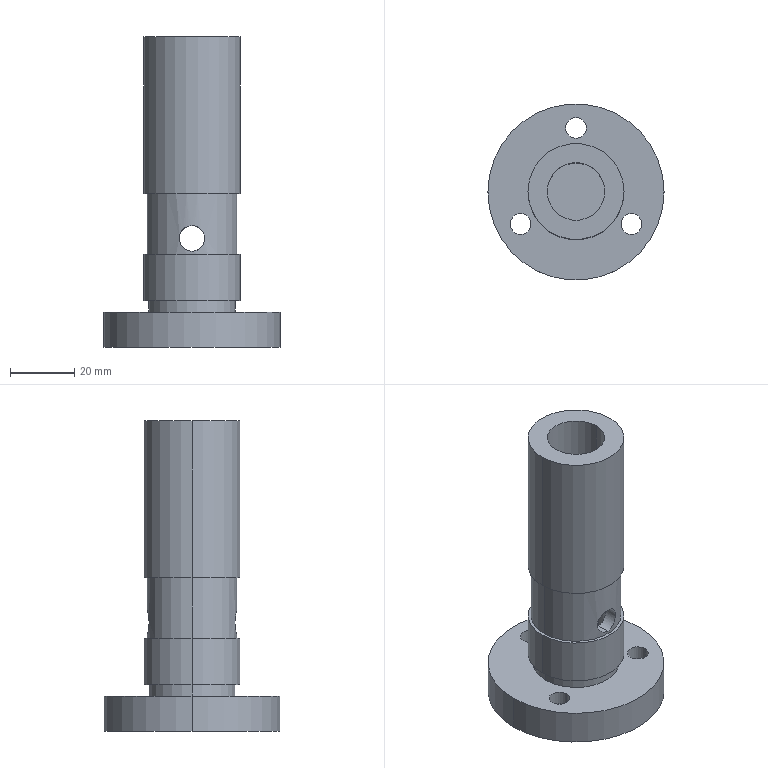Part | SolidWorks | features ICE 9, CirPattern 1, Extrusion 1 | 1 solid | 41 faces | box 55 x 55 x 97 mm | volume 56843 mm3 | cylinder 30 | plane 11 | commonest cylinder face diameters 6.5 x6 11 x6 8 x4 30 x4 18 x2 20 x2
STEP:
#1=CARTESIAN_POINT('',(0.,-14.,30.));
#2=VERTEX_POINT('',#1);
#3=CARTESIAN_POINT('',(0.,-14.,38.));
#4=VERTEX_POINT('',#3);
#5=CARTESIAN_POINT('',(0.,-14.,30.));
#6=CARTESIAN_POINT('',(-0.2619,-14.,30.));
#7=CARTESIAN_POINT('',(-0.524,-13.993,30.026));
#8=CARTESIAN_POINT('',(-1.043,-13.963,30.129));
#9=CARTESIAN_POINT('',(-1.294,-13.942,30.206));
#10=CARTESIAN_POINT('',(-1.776,-13.889,30.406));
#11=CARTESIAN_POINT('',(-2.01,-13.857,30.532));
#12=CARTESIAN_POINT('',(-2.443,-13.787,30.822));
#13=CARTESIAN_POINT('',(-2.643,-13.749,30.987));
#14=CARTESIAN_POINT('',(-3.012,-13.673,31.355));
#15=CARTESIAN_POINT('',(-3.18,-13.635,31.559));
#16=CARTESIAN_POINT('',(-3.468,-13.564,31.991));
#17=CARTESIAN_POINT('',(-3.592,-13.532,32.22));
#18=CARTESIAN_POINT('',(-3.795,-13.476,32.708));
#19=CARTESIAN_POINT('',(-3.871,-13.454,32.958));
#20=CARTESIAN_POINT('',(-3.973,-13.424,33.47));
#21=CARTESIAN_POINT('',(-4.,-13.416,33.736));
#22=CARTESIAN_POINT('',(-4.,-13.416,34.263));
#23=CARTESIAN_POINT('',(-3.974,-13.424,34.524));
#24=CARTESIAN_POINT('',(-3.872,-13.454,35.038));
#25=CARTESIAN_POINT('',(-3.794,-13.477,35.294));
#26=CARTESIAN_POINT('',(-3.594,-13.531,35.776));
#27=CARTESIAN_POINT('',(-3.471,-13.564,36.005));
#28=CARTESIAN_POINT('',(-3.179,-13.635,36.442));
#29=CARTESIAN_POINT('',(-3.013,-13.673,36.644));
#30=CARTESIAN_POINT('',(-2.646,-13.749,37.011));
#31=CARTESIAN_POINT('',(-2.443,-13.787,37.178));
#32=CARTESIAN_POINT('',(-2.008,-13.857,37.469));
#33=CARTESIAN_POINT('',(-1.779,-13.889,37.592));
#34=CARTESIAN_POINT('',(-1.297,-13.942,37.793));
#35=CARTESIAN_POINT('',(-1.042,-13.964,37.871));
#36=CARTESIAN_POINT('',(-0.5273,-13.992,37.974));
#37=CARTESIAN_POINT('',(-0.2657,-14.,38.));
#38=CARTESIAN_POINT('',(0.,-14.,38.));
#39=B_SPLINE_CURVE_WITH_KNOTS('',3,(#5,#6,#7,#8,#9,#10,#11,#12,#13,#14,#15,#16,#17,#18,#19,#20,#21,#22,#23,#24,#25,#26,#27,#28,#29,#30,#31,#32,#33,#34,#35,#36,#37,#38),.UNSPECIFIED.,.F.,.F.,(4,2,2,2,2,2,2,2,2,2,2,2,2,2,2,2,4),(0.01257,0.01336,0.01414,0.01493,0.01571,0.0165,0.01728,0.01807,0.01886,0.01964,0.02043,0.02121,0.022,0.02278,0.02357,0.02435,0.02514),.UNSPECIFIED.);
#40=EDGE_CURVE('',#2,#4,#39,.T.);
#41=ORIENTED_EDGE('',*,*,#40,.F.);
#42=CARTESIAN_POINT('',(0.,-10.,30.));
#43=VERTEX_POINT('',#42);
#44=CARTESIAN_POINT('',(0.,-26.75,30.));
#45=DIRECTION('',(0.,1.,0.));
#46=VECTOR('',#45,1000.);
#47=LINE('',#44,#46);
#48=EDGE_CURVE('',#2,#43,#47,.T.);
#49=ORIENTED_EDGE('',*,*,#48,.T.);
#50=CARTESIAN_POINT('',(0.,-10.,38.));
#51=VERTEX_POINT('',#50);
#52=CARTESIAN_POINT('',(0.,-10.,38.));
#53=CARTESIAN_POINT('',(-0.2673,-10.,38.));
#54=CARTESIAN_POINT('',(-0.5296,-9.989,37.973));
#55=CARTESIAN_POINT('',(-1.045,-9.949,37.87));
#56=CARTESIAN_POINT('',(-1.3,-9.918,37.792));
#57=CARTESIAN_POINT('',(-1.784,-9.843,37.59));
#58=CARTESIAN_POINT('',(-2.013,-9.798,37.467));
#59=CARTESIAN_POINT('',(-2.445,-9.699,37.176));
#60=CARTESIAN_POINT('',(-2.648,-9.645,37.009));
#61=CARTESIAN_POINT('',(-3.013,-9.537,36.644));
#62=CARTESIAN_POINT('',(-3.178,-9.483,36.444));
#63=CARTESIAN_POINT('',(-3.469,-9.38,36.009));
#64=CARTESIAN_POINT('',(-3.591,-9.333,35.78));
#65=CARTESIAN_POINT('',(-3.792,-9.254,35.3));
#66=CARTESIAN_POINT('',(-3.87,-9.221,35.046));
#67=CARTESIAN_POINT('',(-3.974,-9.177,34.528));
#68=CARTESIAN_POINT('',(-4.,-9.165,34.267));
#69=CARTESIAN_POINT('',(-4.,-9.165,33.738));
#70=CARTESIAN_POINT('',(-3.973,-9.177,33.47));
#71=CARTESIAN_POINT('',(-3.87,-9.221,32.955));
#72=CARTESIAN_POINT('',(-3.793,-9.253,32.703));
#73=CARTESIAN_POINT('',(-3.59,-9.334,32.216));
#74=CARTESIAN_POINT('',(-3.466,-9.381,31.987));
#75=CARTESIAN_POINT('',(-3.178,-9.483,31.557));
#76=CARTESIAN_POINT('',(-3.01,-9.538,31.354));
#77=CARTESIAN_POINT('',(-2.644,-9.646,30.988));
#78=CARTESIAN_POINT('',(-2.445,-9.699,30.824));
#79=CARTESIAN_POINT('',(-2.013,-9.798,30.534));
#80=CARTESIAN_POINT('',(-1.78,-9.843,30.408));
#81=CARTESIAN_POINT('',(-1.299,-9.918,30.208));
#82=CARTESIAN_POINT('',(-1.049,-9.948,30.131));
#83=CARTESIAN_POINT('',(-0.5273,-9.99,30.026));
#84=CARTESIAN_POINT('',(-0.2633,-10.,30.));
#85=CARTESIAN_POINT('',(0.,-10.,30.));
#86=B_SPLINE_CURVE_WITH_KNOTS('',3,(#52,#53,#54,#55,#56,#57,#58,#59,#60,#61,#62,#63,#64,#65,#66,#67,#68,#69,#70,#71,#72,#73,#74,#75,#76,#77,#78,#79,#80,#81,#82,#83,#84,#85),.UNSPECIFIED.,.F.,.F.,(4,2,2,2,2,2,2,2,2,2,2,2,2,2,2,2,4),(0.,0.00079,0.00158,0.00237,0.00316,0.00395,0.00474,0.00553,0.00632,0.00711,0.0079,0.00869,0.00948,0.01027,0.01106,0.01185,0.01264),.UNSPECIFIED.);
#87=EDGE_CURVE('',#51,#43,#86,.T.);
#88=ORIENTED_EDGE('',*,*,#87,.F.);
#89=CARTESIAN_POINT('',(0.,-26.75,38.));
#90=DIRECTION('',(0.,1.,0.));
#91=VECTOR('',#90,1000.);
#92=LINE('',#89,#91);
#93=EDGE_CURVE('',#4,#51,#92,.T.);
#94=ORIENTED_EDGE('',*,*,#93,.F.);
#95=EDGE_LOOP('',(#41,#49,#88,#94));
#96=FACE_OUTER_BOUND('',#95,.T.);
#97=CARTESIAN_POINT('',(0.,-26.75,34.));
#98=DIRECTION('',(0.,1.,0.));
#99=DIRECTION('',(0.,0.,1.));
#100=AXIS2_PLACEMENT_3D('',#97,#98,#99);
#101=CYLINDRICAL_SURFACE('',#100,4.);
#102=ADVANCED_FACE('',(#96),#101,.F.);
#103=CARTESIAN_POINT('',(0.,10.,30.));
#104=VERTEX_POINT('',#103);
#105=CARTESIAN_POINT('',(0.,10.,38.));
#106=VERTEX_POINT('',#105);
#107=CARTESIAN_POINT('',(0.,10.,30.));
#108=CARTESIAN_POINT('',(-0.2631,10.,30.));
#109=CARTESIAN_POINT('',(-0.5298,9.989,30.026));
#110=CARTESIAN_POINT('',(-1.048,9.948,30.131));
#111=CARTESIAN_POINT('',(-1.299,9.918,30.208));
#112=CARTESIAN_POINT('',(-1.782,9.843,30.409));
#113=CARTESIAN_POINT('',(-2.015,9.797,30.535));
#114=CARTESIAN_POINT('',(-2.446,9.699,30.824));
#115=CARTESIAN_POINT('',(-2.646,9.645,30.989));
#116=CARTESIAN_POINT('',(-3.015,9.537,31.358));
#117=CARTESIAN_POINT('',(-3.179,9.483,31.558));
#118=CARTESIAN_POINT('',(-3.466,9.381,31.987));
#119=CARTESIAN_POINT('',(-3.592,9.333,32.22));
#120=CARTESIAN_POINT('',(-3.793,9.253,32.703));
#121=CARTESIAN_POINT('',(-3.869,9.221,32.952));
#122=CARTESIAN_POINT('',(-3.973,9.177,33.468));
#123=CARTESIAN_POINT('',(-4.,9.165,33.736));
#124=CARTESIAN_POINT('',(-4.,9.165,34.263));
#125=CARTESIAN_POINT('',(-3.974,9.177,34.525));
#126=CARTESIAN_POINT('',(-3.87,9.221,35.046));
#127=CARTESIAN_POINT('',(-3.792,9.254,35.298));
#128=CARTESIAN_POINT('',(-3.592,9.333,35.78));
#129=CARTESIAN_POINT('',(-3.467,9.381,36.013));
#130=CARTESIAN_POINT('',(-3.177,9.483,36.444));
#131=CARTESIAN_POINT('',(-3.013,9.537,36.644));
#132=CARTESIAN_POINT('',(-2.646,9.645,37.011));
#133=CARTESIAN_POINT('',(-2.443,9.699,37.178));
#134=CARTESIAN_POINT('',(-2.014,9.798,37.466));
#135=CARTESIAN_POINT('',(-1.785,9.842,37.589));
#136=CARTESIAN_POINT('',(-1.298,9.918,37.793));
#137=CARTESIAN_POINT('',(-1.046,9.948,37.87));
#138=CARTESIAN_POINT('',(-0.5323,9.989,37.973));
#139=CARTESIAN_POINT('',(-0.2671,10.,38.));
#140=CARTESIAN_POINT('',(0.,10.,38.));
#141=B_SPLINE_CURVE_WITH_KNOTS('',3,(#107,#108,#109,#110,#111,#112,#113,#114,#115,#116,#117,#118,#119,#120,#121,#122,#123,#124,#125,#126,#127,#128,#129,#130,#131,#132,#133,#134,#135,#136,#137,#138,#139,#140),.UNSPECIFIED.,.F.,.F.,(4,2,2,2,2,2,2,2,2,2,2,2,2,2,2,2,4),(0.01264,0.01343,0.01422,0.01501,0.0158,0.01659,0.01738,0.01817,0.01896,0.01974,0.02053,0.02132,0.02211,0.0229,0.02369,0.02448,0.02527),.UNSPECIFIED.);
#142=EDGE_CURVE('',#104,#106,#141,.T.);
#143=ORIENTED_EDGE('',*,*,#142,.F.);
#144=CARTESIAN_POINT('',(0.,14.,30.));
#145=VERTEX_POINT('',#144);
#146=CARTESIAN_POINT('',(0.,-26.75,30.));
#147=DIRECTION('',(0.,1.,0.));
#148=VECTOR('',#147,1000.);
#149=LINE('',#146,#148);
#150=EDGE_CURVE('',#104,#145,#149,.T.);
#151=ORIENTED_EDGE('',*,*,#150,.T.);
#152=CARTESIAN_POINT('',(0.,14.,38.));
#153=VERTEX_POINT('',#152);
#154=CARTESIAN_POINT('',(0.,14.,38.));
#155=CARTESIAN_POINT('',(-0.2658,14.,38.));
#156=CARTESIAN_POINT('',(-0.5269,13.992,37.974));
#157=CARTESIAN_POINT('',(-1.04,13.964,37.871));
#158=CARTESIAN_POINT('',(-1.295,13.942,37.794));
#159=CARTESIAN_POINT('',(-1.779,13.889,37.592));
#160=CARTESIAN_POINT('',(-2.008,13.857,37.469));
#161=CARTESIAN_POINT('',(-2.442,13.787,37.179));
#162=CARTESIAN_POINT('',(-2.646,13.749,37.011));
#163=CARTESIAN_POINT('',(-3.013,13.673,36.644));
#164=CARTESIAN_POINT('',(-3.178,13.635,36.443));
#165=CARTESIAN_POINT('',(-3.47,13.564,36.007));
#166=CARTESIAN_POINT('',(-3.594,13.531,35.776));
#167=CARTESIAN_POINT('',(-3.793,13.477,35.295));
#168=CARTESIAN_POINT('',(-3.871,13.454,35.042));
#169=CARTESIAN_POINT('',(-3.974,13.424,34.525));
#170=CARTESIAN_POINT('',(-4.,13.416,34.264));
#171=CARTESIAN_POINT('',(-4.,13.416,33.739));
#172=CARTESIAN_POINT('',(-3.974,13.424,33.473));
#173=CARTESIAN_POINT('',(-3.871,13.454,32.958));
#174=CARTESIAN_POINT('',(-3.795,13.476,32.708));
#175=CARTESIAN_POINT('',(-3.593,13.532,32.222));
#176=CARTESIAN_POINT('',(-3.468,13.564,31.991));
#177=CARTESIAN_POINT('',(-3.179,13.635,31.559));
#178=CARTESIAN_POINT('',(-3.012,13.673,31.355));
#179=CARTESIAN_POINT('',(-2.643,13.75,30.986));
#180=CARTESIAN_POINT('',(-2.442,13.787,30.821));
#181=CARTESIAN_POINT('',(-2.01,13.857,30.532));
#182=CARTESIAN_POINT('',(-1.776,13.889,30.406));
#183=CARTESIAN_POINT('',(-1.293,13.942,30.206));
#184=CARTESIAN_POINT('',(-1.044,13.963,30.13));
#185=CARTESIAN_POINT('',(-0.5274,13.992,30.026));
#186=CARTESIAN_POINT('',(-0.2619,14.,30.));
#187=CARTESIAN_POINT('',(0.,14.,30.));
#188=B_SPLINE_CURVE_WITH_KNOTS('',3,(#154,#155,#156,#157,#158,#159,#160,#161,#162,#163,#164,#165,#166,#167,#168,#169,#170,#171,#172,#173,#174,#175,#176,#177,#178,#179,#180,#181,#182,#183,#184,#185,#186,#187),.UNSPECIFIED.,.F.,.F.,(4,2,2,2,2,2,2,2,2,2,2,2,2,2,2,2,4),(0.,0.0007857,0.001571,0.002357,0.003143,0.003929,0.004714,0.0055,0.006286,0.007072,0.007857,0.008643,0.009429,0.01021,0.011,0.01179,0.01257),.UNSPECIFIED.);
#189=EDGE_CURVE('',#153,#145,#188,.T.);
#190=ORIENTED_EDGE('',*,*,#189,.F.);
#191=CARTESIAN_POINT('',(0.,-26.75,38.));
#192=DIRECTION('',(0.,1.,0.));
#193=VECTOR('',#192,1000.);
#194=LINE('',#191,#193);
#195=EDGE_CURVE('',#106,#153,#194,.T.);
#196=ORIENTED_EDGE('',*,*,#195,.F.);
#197=EDGE_LOOP('',(#143,#151,#190,#196));
#198=FACE_OUTER_BOUND('',#197,.T.);
#199=CARTESIAN_POINT('',(0.,-26.75,34.));
#200=DIRECTION('',(0.,1.,0.));
#201=DIRECTION('',(0.,0.,1.));
#202=AXIS2_PLACEMENT_3D('',#199,#200,#201);
#203=CYLINDRICAL_SURFACE('',#202,4.);
#204=ADVANCED_FACE('',(#198),#203,.F.);
#205=CARTESIAN_POINT('',(-20.571,-10.,11.));
#206=VERTEX_POINT('',#205);
#207=CARTESIAN_POINT('',(-14.071,-10.,11.));
#208=VERTEX_POINT('',#207);
#209=CARTESIAN_POINT('',(-17.321,-10.,11.));
#210=DIRECTION('',(0.,0.,1.));
#211=DIRECTION('',(1.,0.,0.));
#212=AXIS2_PLACEMENT_3D('',#209,#210,#211);
#213=CIRCLE('',#212,3.25);
#214=EDGE_CURVE('',#206,#208,#213,.T.);
#215=ORIENTED_EDGE('',*,*,#214,.T.);
#216=CARTESIAN_POINT('',(-14.071,-10.,6.5));
#217=VERTEX_POINT('',#216);
#218=CARTESIAN_POINT('',(-14.071,-10.,13.));
#219=DIRECTION('',(0.,0.,-1.));
#220=VECTOR('',#219,1000.);
#221=LINE('',#218,#220);
#222=EDGE_CURVE('',#208,#217,#221,.T.);
#223=ORIENTED_EDGE('',*,*,#222,.T.);
#224=CARTESIAN_POINT('',(-20.571,-10.,6.5));
#225=VERTEX_POINT('',#224);
#226=CARTESIAN_POINT('',(-17.321,-10.,6.5));
#227=DIRECTION('',(0.,0.,-1.));
#228=DIRECTION('',(0.5,-0.866,0.));
#229=AXIS2_PLACEMENT_3D('',#226,#227,#228);
#230=CIRCLE('',#229,3.25);
#231=EDGE_CURVE('',#217,#225,#230,.T.);
#232=ORIENTED_EDGE('',*,*,#231,.T.);
#233=CARTESIAN_POINT('',(-20.571,-10.,13.));
#234=DIRECTION('',(0.,0.,-1.));
#235=VECTOR('',#234,1000.);
#236=LINE('',#233,#235);
#237=EDGE_CURVE('',#206,#225,#236,.T.);
#238=ORIENTED_EDGE('',*,*,#237,.F.);
#239=EDGE_LOOP('',(#215,#223,#232,#238));
#240=FACE_OUTER_BOUND('',#239,.T.);
#241=CARTESIAN_POINT('',(-17.321,-10.,13.));
#242=DIRECTION('',(0.,0.,-1.));
#243=DIRECTION('',(-1.,0.,0.));
#244=AXIS2_PLACEMENT_3D('',#241,#242,#243);
#245=CYLINDRICAL_SURFACE('',#244,3.25);
#246=ADVANCED_FACE('',(#240),#245,.F.);
#247=CARTESIAN_POINT('',(14.071,-10.,11.));
#248=VERTEX_POINT('',#247);
#249=CARTESIAN_POINT('',(20.571,-10.,11.));
#250=VERTEX_POINT('',#249);
#251=CARTESIAN_POINT('',(17.321,-10.,11.));
#252=DIRECTION('',(0.,0.,1.));
#253=DIRECTION('',(1.,0.,0.));
#254=AXIS2_PLACEMENT_3D('',#251,#252,#253);
#255=CIRCLE('',#254,3.25);
#256=EDGE_CURVE('',#248,#250,#255,.T.);
#257=ORIENTED_EDGE('',*,*,#256,.T.);
#258=CARTESIAN_POINT('',(20.571,-10.,6.5));
#259=VERTEX_POINT('',#258);
#260=CARTESIAN_POINT('',(20.571,-10.,13.));
#261=DIRECTION('',(0.,0.,-1.));
#262=VECTOR('',#261,1000.);
#263=LINE('',#260,#262);
#264=EDGE_CURVE('',#250,#259,#263,.T.);
#265=ORIENTED_EDGE('',*,*,#264,.T.);
#266=CARTESIAN_POINT('',(14.071,-10.,6.5));
#267=VERTEX_POINT('',#266);
#268=CARTESIAN_POINT('',(17.321,-10.,6.5));
#269=DIRECTION('',(0.,0.,-1.));
#270=DIRECTION('',(0.5,0.866,0.));
#271=AXIS2_PLACEMENT_3D('',#268,#269,#270);
#272=CIRCLE('',#271,3.25);
#273=EDGE_CURVE('',#259,#267,#272,.T.);
#274=ORIENTED_EDGE('',*,*,#273,.T.);
#275=CARTESIAN_POINT('',(14.071,-10.,13.));
#276=DIRECTION('',(0.,0.,-1.));
#277=VECTOR('',#276,1000.);
#278=LINE('',#275,#277);
#279=EDGE_CURVE('',#248,#267,#278,.T.);
#280=ORIENTED_EDGE('',*,*,#279,.F.);
#281=EDGE_LOOP('',(#257,#265,#274,#280));
#282=FACE_OUTER_BOUND('',#281,.T.);
#283=CARTESIAN_POINT('',(17.321,-10.,13.));
#284=DIRECTION('',(0.,0.,-1.));
#285=DIRECTION('',(-1.,0.,0.));
#286=AXIS2_PLACEMENT_3D('',#283,#284,#285);
#287=CYLINDRICAL_SURFACE('',#286,3.25);
#288=ADVANCED_FACE('',(#282),#287,.F.);
#289=CARTESIAN_POINT('',(-11.821,-10.,6.5));
#290=VERTEX_POINT('',#289);
#291=CARTESIAN_POINT('',(-22.821,-10.,6.5));
#292=VERTEX_POINT('',#291);
#293=CARTESIAN_POINT('',(-17.321,-10.,6.5));
#294=DIRECTION('',(0.,0.,-1.));
#295=DIRECTION('',(0.5,-0.866,0.));
#296=AXIS2_PLACEMENT_3D('',#293,#294,#295);
#297=CIRCLE('',#296,5.5);
#298=EDGE_CURVE('',#290,#292,#297,.T.);
#299=ORIENTED_EDGE('',*,*,#298,.F.);
#300=CARTESIAN_POINT('',(-11.821,-10.,0.));
#301=VERTEX_POINT('',#300);
#302=CARTESIAN_POINT('',(-11.821,-10.,6.5));
#303=DIRECTION('',(0.,0.,-1.));
#304=VECTOR('',#303,1000.);
#305=LINE('',#302,#304);
#306=EDGE_CURVE('',#290,#301,#305,.T.);
#307=ORIENTED_EDGE('',*,*,#306,.T.);
#308=CARTESIAN_POINT('',(-22.821,-10.,0.));
#309=VERTEX_POINT('',#308);
#310=CARTESIAN_POINT('',(-17.321,-10.,0.));
#311=DIRECTION('',(0.,0.,-1.));
#312=DIRECTION('',(0.5,-0.866,0.));
#313=AXIS2_PLACEMENT_3D('',#310,#311,#312);
#314=CIRCLE('',#313,5.5);
#315=EDGE_CURVE('',#301,#309,#314,.T.);
#316=ORIENTED_EDGE('',*,*,#315,.T.);
#317=CARTESIAN_POINT('',(-22.821,-10.,6.5));
#318=DIRECTION('',(0.,0.,-1.));
#319=VECTOR('',#318,1000.);
#320=LINE('',#317,#319);
#321=EDGE_CURVE('',#292,#309,#320,.T.);
#322=ORIENTED_EDGE('',*,*,#321,.F.);
#323=EDGE_LOOP('',(#299,#307,#316,#322));
#324=FACE_OUTER_BOUND('',#323,.T.);
#325=CARTESIAN_POINT('',(-17.321,-10.,6.5));
#326=DIRECTION('',(0.,0.,-1.));
#327=DIRECTION('',(-1.,0.,0.));
#328=AXIS2_PLACEMENT_3D('',#325,#326,#327);
#329=CYLINDRICAL_SURFACE('',#328,5.5);
#330=ADVANCED_FACE('',(#324),#329,.F.);
#331=CARTESIAN_POINT('',(22.821,-10.,6.5));
#332=VERTEX_POINT('',#331);
#333=CARTESIAN_POINT('',(11.821,-10.,6.5));
#334=VERTEX_POINT('',#333);
#335=CARTESIAN_POINT('',(17.321,-10.,6.5));
#336=DIRECTION('',(0.,0.,-1.));
#337=DIRECTION('',(0.5,0.866,0.));
#338=AXIS2_PLACEMENT_3D('',#335,#336,#337);
#339=CIRCLE('',#338,5.5);
#340=EDGE_CURVE('',#332,#334,#339,.T.);
#341=ORIENTED_EDGE('',*,*,#340,.F.);
#342=CARTESIAN_POINT('',(22.821,-10.,0.));
#343=VERTEX_POINT('',#342);
#344=CARTESIAN_POINT('',(22.821,-10.,6.5));
#345=DIRECTION('',(0.,0.,-1.));
#346=VECTOR('',#345,1000.);
#347=LINE('',#344,#346);
#348=EDGE_CURVE('',#332,#343,#347,.T.);
#349=ORIENTED_EDGE('',*,*,#348,.T.);
#350=CARTESIAN_POINT('',(11.821,-10.,0.));
#351=VERTEX_POINT('',#350);
#352=CARTESIAN_POINT('',(17.321,-10.,0.));
#353=DIRECTION('',(0.,0.,-1.));
#354=DIRECTION('',(0.5,0.866,0.));
#355=AXIS2_PLACEMENT_3D('',#352,#353,#354);
#356=CIRCLE('',#355,5.5);
#357=EDGE_CURVE('',#343,#351,#356,.T.);
#358=ORIENTED_EDGE('',*,*,#357,.T.);
#359=CARTESIAN_POINT('',(11.821,-10.,6.5));
#360=DIRECTION('',(0.,0.,-1.));
#361=VECTOR('',#360,1000.);
#362=LINE('',#359,#361);
#363=EDGE_CURVE('',#334,#351,#362,.T.);
#364=ORIENTED_EDGE('',*,*,#363,.F.);
#365=EDGE_LOOP('',(#341,#349,#358,#364));
#366=FACE_OUTER_BOUND('',#365,.T.);
#367=CARTESIAN_POINT('',(17.321,-10.,6.5));
#368=DIRECTION('',(0.,0.,-1.));
#369=DIRECTION('',(-1.,0.,0.));
#370=AXIS2_PLACEMENT_3D('',#367,#368,#369);
#371=CYLINDRICAL_SURFACE('',#370,5.5);
#372=ADVANCED_FACE('',(#366),#371,.F.);
#373=CARTESIAN_POINT('',(-3.25,20.,11.));
#374=VERTEX_POINT('',#373);
#375=CARTESIAN_POINT('',(3.25,20.,11.));
#376=VERTEX_POINT('',#375);
#377=CARTESIAN_POINT('',(0.,20.,11.));
#378=DIRECTION('',(0.,0.,1.));
#379=DIRECTION('',(1.,0.,0.));
#380=AXIS2_PLACEMENT_3D('',#377,#378,#379);
#381=CIRCLE('',#380,3.25);
#382=EDGE_CURVE('',#374,#376,#381,.T.);
#383=ORIENTED_EDGE('',*,*,#382,.T.);
#384=CARTESIAN_POINT('',(3.25,20.,6.5));
#385=VERTEX_POINT('',#384);
#386=CARTESIAN_POINT('',(3.25,20.,13.));
#387=DIRECTION('',(0.,0.,-1.));
#388=VECTOR('',#387,1000.);
#389=LINE('',#386,#388);
#390=EDGE_CURVE('',#376,#385,#389,.T.);
#391=ORIENTED_EDGE('',*,*,#390,.T.);
#392=CARTESIAN_POINT('',(-3.25,20.,6.5));
#393=VERTEX_POINT('',#392);
#394=CARTESIAN_POINT('',(0.,20.,6.5));
#395=DIRECTION('',(0.,0.,-1.));
#396=DIRECTION('',(-1.,0.,0.));
#397=AXIS2_PLACEMENT_3D('',#394,#395,#396);
#398=CIRCLE('',#397,3.25);
#399=EDGE_CURVE('',#385,#393,#398,.T.);
#400=ORIENTED_EDGE('',*,*,#399,.T.);
#401=CARTESIAN_POINT('',(-3.25,20.,13.));
#402=DIRECTION('',(0.,0.,-1.));
#403=VECTOR('',#402,1000.);
#404=LINE('',#401,#403);
#405=EDGE_CURVE('',#374,#393,#404,.T.);
#406=ORIENTED_EDGE('',*,*,#405,.F.);
#407=EDGE_LOOP('',(#383,#391,#400,#406));
#408=FACE_OUTER_BOUND('',#407,.T.);
#409=CARTESIAN_POINT('',(0.,20.,13.));
#410=DIRECTION('',(0.,0.,-1.));
#411=DIRECTION('',(-1.,0.,0.));
#412=AXIS2_PLACEMENT_3D('',#409,#410,#411);
#413=CYLINDRICAL_SURFACE('',#412,3.25);
#414=ADVANCED_FACE('',(#408),#413,.F.);
#415=CARTESIAN_POINT('',(5.5,20.,6.5));
#416=VERTEX_POINT('',#415);
#417=CARTESIAN_POINT('',(-5.5,20.,6.5));
#418=VERTEX_POINT('',#417);
#419=CARTESIAN_POINT('',(0.,20.,6.5));
#420=DIRECTION('',(0.,0.,-1.));
#421=DIRECTION('',(-1.,0.,0.));
#422=AXIS2_PLACEMENT_3D('',#419,#420,#421);
#423=CIRCLE('',#422,5.5);
#424=EDGE_CURVE('',#416,#418,#423,.T.);
#425=ORIENTED_EDGE('',*,*,#424,.F.);
#426=CARTESIAN_POINT('',(5.5,20.,0.));
#427=VERTEX_POINT('',#426);
#428=CARTESIAN_POINT('',(5.5,20.,6.5));
#429=DIRECTION('',(0.,0.,-1.));
#430=VECTOR('',#429,1000.);
#431=LINE('',#428,#430);
#432=EDGE_CURVE('',#416,#427,#431,.T.);
#433=ORIENTED_EDGE('',*,*,#432,.T.);
#434=CARTESIAN_POINT('',(-5.5,20.,0.));
#435=VERTEX_POINT('',#434);
#436=CARTESIAN_POINT('',(0.,20.,0.));
#437=DIRECTION('',(0.,0.,-1.));
#438=DIRECTION('',(-1.,0.,0.));
#439=AXIS2_PLACEMENT_3D('',#436,#437,#438);
#440=CIRCLE('',#439,5.5);
#441=EDGE_CURVE('',#427,#435,#440,.T.);
#442=ORIENTED_EDGE('',*,*,#441,.T.);
#443=CARTESIAN_POINT('',(-5.5,20.,6.5));
#444=DIRECTION('',(0.,0.,-1.));
#445=VECTOR('',#444,1000.);
#446=LINE('',#443,#445);
#447=EDGE_CURVE('',#418,#435,#446,.T.);
#448=ORIENTED_EDGE('',*,*,#447,.F.);
#449=EDGE_LOOP('',(#425,#433,#442,#448));
#450=FACE_OUTER_BOUND('',#449,.T.);
#451=CARTESIAN_POINT('',(0.,20.,6.5));
#452=DIRECTION('',(0.,0.,-1.));
#453=DIRECTION('',(-1.,0.,0.));
#454=AXIS2_PLACEMENT_3D('',#451,#452,#453);
#455=CYLINDRICAL_SURFACE('',#454,5.5);
#456=ADVANCED_FACE('',(#450),#455,.F.);
#457=ORIENTED_EDGE('',*,*,#87,.T.);
#458=CARTESIAN_POINT('',(0.,-10.,30.));
#459=CARTESIAN_POINT('',(0.2631,-10.,30.));
#460=CARTESIAN_POINT('',(0.5298,-9.989,30.026));
#461=CARTESIAN_POINT('',(1.048,-9.948,30.131));
#462=CARTESIAN_POINT('',(1.299,-9.918,30.208));
#463=CARTESIAN_POINT('',(1.782,-9.843,30.409));
#464=CARTESIAN_POINT('',(2.015,-9.797,30.535));
#465=CARTESIAN_POINT('',(2.446,-9.699,30.824));
#466=CARTESIAN_POINT('',(2.646,-9.645,30.989));
#467=CARTESIAN_POINT('',(3.015,-9.537,31.358));
#468=CARTESIAN_POINT('',(3.179,-9.483,31.558));
#469=CARTESIAN_POINT('',(3.466,-9.381,31.987));
#470=CARTESIAN_POINT('',(3.592,-9.333,32.22));
#471=CARTESIAN_POINT('',(3.793,-9.253,32.703));
#472=CARTESIAN_POINT('',(3.869,-9.221,32.952));
#473=CARTESIAN_POINT('',(3.973,-9.177,33.468));
#474=CARTESIAN_POINT('',(4.,-9.165,33.736));
#475=CARTESIAN_POINT('',(4.,-9.165,34.263));
#476=CARTESIAN_POINT('',(3.974,-9.177,34.525));
#477=CARTESIAN_POINT('',(3.87,-9.221,35.046));
#478=CARTESIAN_POINT('',(3.792,-9.254,35.298));
#479=CARTESIAN_POINT('',(3.592,-9.333,35.78));
#480=CARTESIAN_POINT('',(3.467,-9.381,36.013));
#481=CARTESIAN_POINT('',(3.177,-9.483,36.444));
#482=CARTESIAN_POINT('',(3.013,-9.537,36.644));
#483=CARTESIAN_POINT('',(2.646,-9.645,37.011));
#484=CARTESIAN_POINT('',(2.443,-9.699,37.178));
#485=CARTESIAN_POINT('',(2.014,-9.798,37.466));
#486=CARTESIAN_POINT('',(1.785,-9.842,37.589));
#487=CARTESIAN_POINT('',(1.298,-9.918,37.793));
#488=CARTESIAN_POINT('',(1.046,-9.948,37.87));
#489=CARTESIAN_POINT('',(0.5323,-9.989,37.973));
#490=CARTESIAN_POINT('',(0.2671,-10.,38.));
#491=CARTESIAN_POINT('',(0.,-10.,38.));
#492=B_SPLINE_CURVE_WITH_KNOTS('',3,(#458,#459,#460,#461,#462,#463,#464,#465,#466,#467,#468,#469,#470,#471,#472,#473,#474,#475,#476,#477,#478,#479,#480,#481,#482,#483,#484,#485,#486,#487,#488,#489,#490,#491),.UNSPECIFIED.,.F.,.F.,(4,2,2,2,2,2,2,2,2,2,2,2,2,2,2,2,4),(0.01264,0.01343,0.01422,0.01501,0.0158,0.01659,0.01738,0.01817,0.01896,0.01974,0.02053,0.02132,0.02211,0.0229,0.02369,0.02448,0.02527),.UNSPECIFIED.);
#493=EDGE_CURVE('',#43,#51,#492,.T.);
#494=ORIENTED_EDGE('',*,*,#493,.T.);
#495=EDGE_LOOP('',(#457,#494));
#496=FACE_BOUND('',#495,.T.);
#497=CARTESIAN_POINT('',(-10.,0.,7.));
#498=VERTEX_POINT('',#497);
#499=CARTESIAN_POINT('',(10.,0.,7.));
#500=VERTEX_POINT('',#499);
#501=CARTESIAN_POINT('',(0.,0.,7.));
#502=DIRECTION('',(0.,0.,1.));
#503=DIRECTION('',(1.,0.,0.));
#504=AXIS2_PLACEMENT_3D('',#501,#502,#503);
#505=CIRCLE('',#504,10.);
#506=EDGE_CURVE('',#498,#500,#505,.T.);
#507=ORIENTED_EDGE('',*,*,#506,.F.);
#508=CARTESIAN_POINT('',(-10.,0.,45.));
#509=VERTEX_POINT('',#508);
#510=CARTESIAN_POINT('',(-10.,0.,7.));
#511=DIRECTION('',(0.,0.,1.));
#512=VECTOR('',#511,1000.);
#513=LINE('',#510,#512);
#514=EDGE_CURVE('',#498,#509,#513,.T.);
#515=ORIENTED_EDGE('',*,*,#514,.T.);
#516=CARTESIAN_POINT('',(10.,0.,45.));
#517=VERTEX_POINT('',#516);
#518=CARTESIAN_POINT('',(0.,0.,45.));
#519=DIRECTION('',(0.,0.,1.));
#520=DIRECTION('',(1.,0.,0.));
#521=AXIS2_PLACEMENT_3D('',#518,#519,#520);
#522=CIRCLE('',#521,10.);
#523=EDGE_CURVE('',#509,#517,#522,.T.);
#524=ORIENTED_EDGE('',*,*,#523,.T.);
#525=CARTESIAN_POINT('',(10.,0.,7.));
#526=DIRECTION('',(0.,0.,1.));
#527=VECTOR('',#526,1000.);
#528=LINE('',#525,#527);
#529=EDGE_CURVE('',#500,#517,#528,.T.);
#530=ORIENTED_EDGE('',*,*,#529,.F.);
#531=EDGE_LOOP('',(#507,#515,#524,#530));
#532=FACE_OUTER_BOUND('',#531,.T.);
#533=CARTESIAN_POINT('',(0.,0.,7.));
#534=DIRECTION('',(0.,0.,1.));
#535=DIRECTION('',(1.,0.,0.));
#536=AXIS2_PLACEMENT_3D('',#533,#534,#535);
#537=CYLINDRICAL_SURFACE('',#536,10.);
#538=ADVANCED_FACE('',(#496,#532),#537,.F.);
#539=CARTESIAN_POINT('',(-9.,0.,45.));
#540=VERTEX_POINT('',#539);
#541=CARTESIAN_POINT('',(9.,0.,45.));
#542=VERTEX_POINT('',#541);
#543=CARTESIAN_POINT('',(0.,0.,45.));
#544=DIRECTION('',(0.,0.,1.));
#545=DIRECTION('',(1.,0.,0.));
#546=AXIS2_PLACEMENT_3D('',#543,#544,#545);
#547=CIRCLE('',#546,9.);
#548=EDGE_CURVE('',#540,#542,#547,.T.);
#549=ORIENTED_EDGE('',*,*,#548,.F.);
#550=CARTESIAN_POINT('',(-9.,0.,97.));
#551=VERTEX_POINT('',#550);
#552=CARTESIAN_POINT('',(-9.,0.,45.));
#553=DIRECTION('',(0.,0.,1.));
#554=VECTOR('',#553,1000.);
#555=LINE('',#552,#554);
#556=EDGE_CURVE('',#540,#551,#555,.T.);
#557=ORIENTED_EDGE('',*,*,#556,.T.);
#558=CARTESIAN_POINT('',(9.,0.,97.));
#559=VERTEX_POINT('',#558);
#560=CARTESIAN_POINT('',(0.,0.,97.));
#561=DIRECTION('',(0.,0.,1.));
#562=DIRECTION('',(1.,0.,0.));
#563=AXIS2_PLACEMENT_3D('',#560,#561,#562);
#564=CIRCLE('',#563,9.);
#565=EDGE_CURVE('',#551,#559,#564,.T.);
#566=ORIENTED_EDGE('',*,*,#565,.T.);
#567=CARTESIAN_POINT('',(9.,0.,45.));
#568=DIRECTION('',(0.,0.,1.));
#569=VECTOR('',#568,1000.);
#570=LINE('',#567,#569);
#571=EDGE_CURVE('',#542,#559,#570,.T.);
#572=ORIENTED_EDGE('',*,*,#571,.F.);
#573=EDGE_LOOP('',(#549,#557,#566,#572));
#574=FACE_OUTER_BOUND('',#573,.T.);
#575=CARTESIAN_POINT('',(0.,0.,45.));
#576=DIRECTION('',(0.,0.,1.));
#577=DIRECTION('',(1.,0.,0.));
#578=AXIS2_PLACEMENT_3D('',#575,#576,#577);
#579=CYLINDRICAL_SURFACE('',#578,9.);
#580=ADVANCED_FACE('',(#574),#579,.F.);
#581=CARTESIAN_POINT('',(15.,0.,97.));
#582=VERTEX_POINT('',#581);
#583=CARTESIAN_POINT('',(-15.,0.,97.));
#584=VERTEX_POINT('',#583);
#585=CARTESIAN_POINT('',(0.,0.,97.));
#586=DIRECTION('',(0.,0.,1.));
#587=DIRECTION('',(1.,0.,0.));
#588=AXIS2_PLACEMENT_3D('',#585,#586,#587);
#589=CIRCLE('',#588,15.);
#590=EDGE_CURVE('',#582,#584,#589,.T.);
#591=ORIENTED_EDGE('',*,*,#590,.F.);
#592=CARTESIAN_POINT('',(15.,0.,48.));
#593=VERTEX_POINT('',#592);
#594=CARTESIAN_POINT('',(15.,0.,97.));
#595=DIRECTION('',(0.,0.,-1.));
#596=VECTOR('',#595,1000.);
#597=LINE('',#594,#596);
#598=EDGE_CURVE('',#582,#593,#597,.T.);
#599=ORIENTED_EDGE('',*,*,#598,.T.);
#600=CARTESIAN_POINT('',(-15.,0.,48.));
#601=VERTEX_POINT('',#600);
#602=CARTESIAN_POINT('',(0.,0.,48.));
#603=DIRECTION('',(0.,0.,1.));
#604=DIRECTION('',(1.,0.,0.));
#605=AXIS2_PLACEMENT_3D('',#602,#603,#604);
#606=CIRCLE('',#605,15.);
#607=EDGE_CURVE('',#593,#601,#606,.T.);
#608=ORIENTED_EDGE('',*,*,#607,.T.);
#609=CARTESIAN_POINT('',(-15.,0.,97.));
#610=DIRECTION('',(0.,0.,-1.));
#611=VECTOR('',#610,1000.);
#612=LINE('',#609,#611);
#613=EDGE_CURVE('',#584,#601,#612,.T.);
#614=ORIENTED_EDGE('',*,*,#613,.F.);
#615=EDGE_LOOP('',(#591,#599,#608,#614));
#616=FACE_OUTER_BOUND('',#615,.T.);
#617=CARTESIAN_POINT('',(0.,0.,97.));
#618=DIRECTION('',(0.,0.,-1.));
#619=DIRECTION('',(-1.,0.,0.));
#620=AXIS2_PLACEMENT_3D('',#617,#618,#619);
#621=CYLINDRICAL_SURFACE('',#620,15.);
#622=ADVANCED_FACE('',(#616),#621,.T.);
#623=ORIENTED_EDGE('',*,*,#189,.T.);
#624=CARTESIAN_POINT('',(0.,14.,30.));
#625=CARTESIAN_POINT('',(0.2619,14.,30.));
#626=CARTESIAN_POINT('',(0.524,13.993,30.026));
#627=CARTESIAN_POINT('',(1.043,13.963,30.129));
#628=CARTESIAN_POINT('',(1.294,13.942,30.206));
#629=CARTESIAN_POINT('',(1.776,13.889,30.406));
#630=CARTESIAN_POINT('',(2.01,13.857,30.532));
#631=CARTESIAN_POINT('',(2.443,13.787,30.822));
#632=CARTESIAN_POINT('',(2.643,13.749,30.987));
#633=CARTESIAN_POINT('',(3.012,13.673,31.355));
#634=CARTESIAN_POINT('',(3.18,13.635,31.559));
#635=CARTESIAN_POINT('',(3.468,13.564,31.991));
#636=CARTESIAN_POINT('',(3.592,13.532,32.22));
#637=CARTESIAN_POINT('',(3.795,13.476,32.708));
#638=CARTESIAN_POINT('',(3.871,13.454,32.958));
#639=CARTESIAN_POINT('',(3.973,13.424,33.47));
#640=CARTESIAN_POINT('',(4.,13.416,33.736));
#641=CARTESIAN_POINT('',(4.,13.416,34.263));
#642=CARTESIAN_POINT('',(3.974,13.424,34.524));
#643=CARTESIAN_POINT('',(3.872,13.454,35.038));
#644=CARTESIAN_POINT('',(3.794,13.477,35.294));
#645=CARTESIAN_POINT('',(3.594,13.531,35.776));
#646=CARTESIAN_POINT('',(3.471,13.564,36.005));
#647=CARTESIAN_POINT('',(3.179,13.635,36.442));
#648=CARTESIAN_POINT('',(3.013,13.673,36.644));
#649=CARTESIAN_POINT('',(2.646,13.749,37.011));
#650=CARTESIAN_POINT('',(2.443,13.787,37.178));
#651=CARTESIAN_POINT('',(2.008,13.857,37.469));
#652=CARTESIAN_POINT('',(1.779,13.889,37.592));
#653=CARTESIAN_POINT('',(1.297,13.942,37.793));
#654=CARTESIAN_POINT('',(1.042,13.964,37.871));
#655=CARTESIAN_POINT('',(0.5273,13.992,37.974));
#656=CARTESIAN_POINT('',(0.2657,14.,38.));
#657=CARTESIAN_POINT('',(0.,14.,38.));
#658=B_SPLINE_CURVE_WITH_KNOTS('',3,(#624,#625,#626,#627,#628,#629,#630,#631,#632,#633,#634,#635,#636,#637,#638,#639,#640,#641,#642,#643,#644,#645,#646,#647,#648,#649,#650,#651,#652,#653,#654,#655,#656,#657),.UNSPECIFIED.,.F.,.F.,(4,2,2,2,2,2,2,2,2,2,2,2,2,2,2,2,4),(0.01257,0.01336,0.01414,0.01493,0.01571,0.0165,0.01728,0.01807,0.01886,0.01964,0.02043,0.02121,0.022,0.02278,0.02357,0.02435,0.02514),.UNSPECIFIED.);
#659=EDGE_CURVE('',#145,#153,#658,.T.);
#660=ORIENTED_EDGE('',*,*,#659,.T.);
#661=EDGE_LOOP('',(#623,#660));
#662=FACE_BOUND('',#661,.T.);
#663=CARTESIAN_POINT('',(14.,0.,48.));
#664=VERTEX_POINT('',#663);
#665=CARTESIAN_POINT('',(-14.,0.,48.));
#666=VERTEX_POINT('',#665);
#667=CARTESIAN_POINT('',(0.,0.,48.));
#668=DIRECTION('',(0.,0.,1.));
#669=DIRECTION('',(1.,0.,0.));
#670=AXIS2_PLACEMENT_3D('',#667,#668,#669);
#671=CIRCLE('',#670,14.);
#672=EDGE_CURVE('',#664,#666,#671,.T.);
#673=ORIENTED_EDGE('',*,*,#672,.F.);
#674=CARTESIAN_POINT('',(14.,0.,29.));
#675=VERTEX_POINT('',#674);
#676=CARTESIAN_POINT('',(14.,0.,48.));
#677=DIRECTION('',(0.,0.,-1.));
#678=VECTOR('',#677,1000.);
#679=LINE('',#676,#678);
#680=EDGE_CURVE('',#664,#675,#679,.T.);
#681=ORIENTED_EDGE('',*,*,#680,.T.);
#682=CARTESIAN_POINT('',(-14.,0.,29.));
#683=VERTEX_POINT('',#682);
#684=CARTESIAN_POINT('',(0.,0.,29.));
#685=DIRECTION('',(0.,0.,1.));
#686=DIRECTION('',(1.,0.,0.));
#687=AXIS2_PLACEMENT_3D('',#684,#685,#686);
#688=CIRCLE('',#687,14.);
#689=EDGE_CURVE('',#675,#683,#688,.T.);
#690=ORIENTED_EDGE('',*,*,#689,.T.);
#691=CARTESIAN_POINT('',(-14.,0.,48.));
#692=DIRECTION('',(0.,0.,-1.));
#693=VECTOR('',#692,1000.);
#694=LINE('',#691,#693);
#695=EDGE_CURVE('',#666,#683,#694,.T.);
#696=ORIENTED_EDGE('',*,*,#695,.F.);
#697=EDGE_LOOP('',(#673,#681,#690,#696));
#698=FACE_OUTER_BOUND('',#697,.T.);
#699=CARTESIAN_POINT('',(0.,0.,48.));
#700=DIRECTION('',(0.,0.,-1.));
#701=DIRECTION('',(-1.,0.,0.));
#702=AXIS2_PLACEMENT_3D('',#699,#700,#701);
#703=CYLINDRICAL_SURFACE('',#702,14.);
#704=ADVANCED_FACE('',(#662,#698),#703,.T.);
#705=CARTESIAN_POINT('',(15.,0.,29.));
#706=VERTEX_POINT('',#705);
#707=CARTESIAN_POINT('',(-15.,0.,29.));
#708=VERTEX_POINT('',#707);
#709=CARTESIAN_POINT('',(0.,0.,29.));
#710=DIRECTION('',(0.,0.,1.));
#711=DIRECTION('',(1.,0.,0.));
#712=AXIS2_PLACEMENT_3D('',#709,#710,#711);
#713=CIRCLE('',#712,15.);
#714=EDGE_CURVE('',#706,#708,#713,.T.);
#715=ORIENTED_EDGE('',*,*,#714,.F.);
#716=CARTESIAN_POINT('',(15.,0.,14.5));
#717=VERTEX_POINT('',#716);
#718=CARTESIAN_POINT('',(15.,0.,29.));
#719=DIRECTION('',(0.,0.,-1.));
#720=VECTOR('',#719,1000.);
#721=LINE('',#718,#720);
#722=EDGE_CURVE('',#706,#717,#721,.T.);
#723=ORIENTED_EDGE('',*,*,#722,.T.);
#724=CARTESIAN_POINT('',(-15.,0.,14.5));
#725=VERTEX_POINT('',#724);
#726=CARTESIAN_POINT('',(0.,0.,14.5));
#727=DIRECTION('',(0.,0.,1.));
#728=DIRECTION('',(1.,0.,0.));
#729=AXIS2_PLACEMENT_3D('',#726,#727,#728);
#730=CIRCLE('',#729,15.);
#731=EDGE_CURVE('',#717,#725,#730,.T.);
#732=ORIENTED_EDGE('',*,*,#731,.T.);
#733=CARTESIAN_POINT('',(-15.,0.,29.));
#734=DIRECTION('',(0.,0.,-1.));
#735=VECTOR('',#734,1000.);
#736=LINE('',#733,#735);
#737=EDGE_CURVE('',#708,#725,#736,.T.);
#738=ORIENTED_EDGE('',*,*,#737,.F.);
#739=EDGE_LOOP('',(#715,#723,#732,#738));
#740=FACE_OUTER_BOUND('',#739,.T.);
#741=CARTESIAN_POINT('',(0.,0.,29.));
#742=DIRECTION('',(0.,0.,-1.));
#743=DIRECTION('',(-1.,0.,0.));
#744=AXIS2_PLACEMENT_3D('',#741,#742,#743);
#745=CYLINDRICAL_SURFACE('',#744,15.);
#746=ADVANCED_FACE('',(#740),#745,.T.);
#747=CARTESIAN_POINT('',(13.5,0.,14.5));
#748=VERTEX_POINT('',#747);
#749=CARTESIAN_POINT('',(-13.5,0.,14.5));
#750=VERTEX_POINT('',#749);
#751=CARTESIAN_POINT('',(0.,0.,14.5));
#752=DIRECTION('',(0.,0.,1.));
#753=DIRECTION('',(1.,0.,0.));
#754=AXIS2_PLACEMENT_3D('',#751,#752,#753);
#755=CIRCLE('',#754,13.5);
#756=EDGE_CURVE('',#748,#750,#755,.T.);
#757=ORIENTED_EDGE('',*,*,#756,.F.);
#758=CARTESIAN_POINT('',(13.5,0.,11.));
#759=VERTEX_POINT('',#758);
#760=CARTESIAN_POINT('',(13.5,0.,14.5));
#761=DIRECTION('',(0.,0.,-1.));
#762=VECTOR('',#761,1000.);
#763=LINE('',#760,#762);
#764=EDGE_CURVE('',#748,#759,#763,.T.);
#765=ORIENTED_EDGE('',*,*,#764,.T.);
#766=CARTESIAN_POINT('',(-13.5,0.,11.));
#767=VERTEX_POINT('',#766);
#768=CARTESIAN_POINT('',(0.,0.,11.));
#769=DIRECTION('',(0.,0.,1.));
#770=DIRECTION('',(1.,0.,0.));
#771=AXIS2_PLACEMENT_3D('',#768,#769,#770);
#772=CIRCLE('',#771,13.5);
#773=EDGE_CURVE('',#759,#767,#772,.T.);
#774=ORIENTED_EDGE('',*,*,#773,.T.);
#775=CARTESIAN_POINT('',(-13.5,0.,14.5));
#776=DIRECTION('',(0.,0.,-1.));
#777=VECTOR('',#776,1000.);
#778=LINE('',#775,#777);
#779=EDGE_CURVE('',#750,#767,#778,.T.);
#780=ORIENTED_EDGE('',*,*,#779,.F.);
#781=EDGE_LOOP('',(#757,#765,#774,#780));
#782=FACE_OUTER_BOUND('',#781,.T.);
#783=CARTESIAN_POINT('',(0.,0.,14.5));
#784=DIRECTION('',(0.,0.,-1.));
#785=DIRECTION('',(-1.,0.,0.));
#786=AXIS2_PLACEMENT_3D('',#783,#784,#785);
#787=CYLINDRICAL_SURFACE('',#786,13.5);
#788=ADVANCED_FACE('',(#782),#787,.T.);
#789=CARTESIAN_POINT('',(27.5,0.,11.));
#790=VERTEX_POINT('',#789);
#791=CARTESIAN_POINT('',(-27.5,0.,11.));
#792=VERTEX_POINT('',#791);
#793=CARTESIAN_POINT('',(0.,0.,11.));
#794=DIRECTION('',(0.,0.,1.));
#795=DIRECTION('',(1.,0.,0.));
#796=AXIS2_PLACEMENT_3D('',#793,#794,#795);
#797=CIRCLE('',#796,27.5);
#798=EDGE_CURVE('',#790,#792,#797,.T.);
#799=ORIENTED_EDGE('',*,*,#798,.F.);
#800=CARTESIAN_POINT('',(27.5,0.,0.));
#801=VERTEX_POINT('',#800);
#802=CARTESIAN_POINT('',(27.5,0.,11.));
#803=DIRECTION('',(0.,0.,-1.));
#804=VECTOR('',#803,1000.);
#805=LINE('',#802,#804);
#806=EDGE_CURVE('',#790,#801,#805,.T.);
#807=ORIENTED_EDGE('',*,*,#806,.T.);
#808=CARTESIAN_POINT('',(-27.5,0.,0.));
#809=VERTEX_POINT('',#808);
#810=CARTESIAN_POINT('',(0.,0.,0.));
#811=DIRECTION('',(0.,0.,1.));
#812=DIRECTION('',(1.,0.,0.));
#813=AXIS2_PLACEMENT_3D('',#810,#811,#812);
#814=CIRCLE('',#813,27.5);
#815=EDGE_CURVE('',#801,#809,#814,.T.);
#816=ORIENTED_EDGE('',*,*,#815,.T.);
#817=CARTESIAN_POINT('',(-27.5,0.,11.));
#818=DIRECTION('',(0.,0.,-1.));
#819=VECTOR('',#818,1000.);
#820=LINE('',#817,#819);
#821=EDGE_CURVE('',#792,#809,#820,.T.);
#822=ORIENTED_EDGE('',*,*,#821,.F.);
#823=EDGE_LOOP('',(#799,#807,#816,#822));
#824=FACE_OUTER_BOUND('',#823,.T.);
#825=CARTESIAN_POINT('',(0.,0.,11.));
#826=DIRECTION('',(0.,0.,-1.));
#827=DIRECTION('',(-1.,0.,0.));
#828=AXIS2_PLACEMENT_3D('',#825,#826,#827);
#829=CYLINDRICAL_SURFACE('',#828,27.5);
#830=ADVANCED_FACE('',(#824),#829,.T.);
#831=ORIENTED_EDGE('',*,*,#806,.F.);
#832=CARTESIAN_POINT('',(0.,0.,11.));
#833=DIRECTION('',(0.,0.,1.));
#834=DIRECTION('',(1.,0.,0.));
#835=AXIS2_PLACEMENT_3D('',#832,#833,#834);
#836=CIRCLE('',#835,27.5);
#837=EDGE_CURVE('',#792,#790,#836,.T.);
#838=ORIENTED_EDGE('',*,*,#837,.F.);
#839=ORIENTED_EDGE('',*,*,#821,.T.);
#840=CARTESIAN_POINT('',(0.,0.,0.));
#841=DIRECTION('',(0.,0.,1.));
#842=DIRECTION('',(1.,0.,0.));
#843=AXIS2_PLACEMENT_3D('',#840,#841,#842);
#844=CIRCLE('',#843,27.5);
#845=EDGE_CURVE('',#809,#801,#844,.T.);
#846=ORIENTED_EDGE('',*,*,#845,.T.);
#847=EDGE_LOOP('',(#831,#838,#839,#846));
#848=FACE_OUTER_BOUND('',#847,.T.);
#849=CARTESIAN_POINT('',(0.,0.,11.));
#850=DIRECTION('',(0.,0.,-1.));
#851=DIRECTION('',(-1.,0.,0.));
#852=AXIS2_PLACEMENT_3D('',#849,#850,#851);
#853=CYLINDRICAL_SURFACE('',#852,27.5);
#854=ADVANCED_FACE('',(#848),#853,.T.);
#855=ORIENTED_EDGE('',*,*,#214,.F.);
#856=CARTESIAN_POINT('',(-17.321,-10.,11.));
#857=DIRECTION('',(0.,0.,1.));
#858=DIRECTION('',(1.,0.,0.));
#859=AXIS2_PLACEMENT_3D('',#856,#857,#858);
#860=CIRCLE('',#859,3.25);
#861=EDGE_CURVE('',#208,#206,#860,.T.);
#862=ORIENTED_EDGE('',*,*,#861,.F.);
#863=EDGE_LOOP('',(#855,#862));
#864=FACE_BOUND('',#863,.T.);
#865=ORIENTED_EDGE('',*,*,#256,.F.);
#866=CARTESIAN_POINT('',(17.321,-10.,11.));
#867=DIRECTION('',(0.,0.,1.));
#868=DIRECTION('',(1.,0.,0.));
#869=AXIS2_PLACEMENT_3D('',#866,#867,#868);
#870=CIRCLE('',#869,3.25);
#871=EDGE_CURVE('',#250,#248,#870,.T.);
#872=ORIENTED_EDGE('',*,*,#871,.F.);
#873=EDGE_LOOP('',(#865,#872));
#874=FACE_BOUND('',#873,.T.);
#875=ORIENTED_EDGE('',*,*,#382,.F.);
#876=CARTESIAN_POINT('',(0.,20.,11.));
#877=DIRECTION('',(0.,0.,1.));
#878=DIRECTION('',(1.,0.,0.));
#879=AXIS2_PLACEMENT_3D('',#876,#877,#878);
#880=CIRCLE('',#879,3.25);
#881=EDGE_CURVE('',#376,#374,#880,.T.);
#882=ORIENTED_EDGE('',*,*,#881,.F.);
#883=EDGE_LOOP('',(#875,#882));
#884=FACE_BOUND('',#883,.T.);
#885=CARTESIAN_POINT('',(0.,0.,11.));
#886=DIRECTION('',(0.,0.,1.));
#887=DIRECTION('',(1.,0.,0.));
#888=AXIS2_PLACEMENT_3D('',#885,#886,#887);
#889=CIRCLE('',#888,13.5);
#890=EDGE_CURVE('',#767,#759,#889,.T.);
#891=ORIENTED_EDGE('',*,*,#890,.F.);
#892=ORIENTED_EDGE('',*,*,#773,.F.);
#893=EDGE_LOOP('',(#891,#892));
#894=FACE_BOUND('',#893,.T.);
#895=ORIENTED_EDGE('',*,*,#837,.T.);
#896=ORIENTED_EDGE('',*,*,#798,.T.);
#897=EDGE_LOOP('',(#895,#896));
#898=FACE_OUTER_BOUND('',#897,.T.);
#899=CARTESIAN_POINT('',(0.,0.,11.));
#900=DIRECTION('',(0.,0.,1.));
#901=DIRECTION('',(1.,0.,0.));
#902=AXIS2_PLACEMENT_3D('',#899,#900,#901);
#903=PLANE('',#902);
#904=ADVANCED_FACE('',(#864,#874,#884,#894,#898),#903,.T.);
#905=CARTESIAN_POINT('',(-17.321,-10.,0.));
#906=DIRECTION('',(0.,0.,-1.));
#907=DIRECTION('',(0.5,-0.866,0.));
#908=AXIS2_PLACEMENT_3D('',#905,#906,#907);
#909=CIRCLE('',#908,5.5);
#910=EDGE_CURVE('',#309,#301,#909,.T.);
#911=ORIENTED_EDGE('',*,*,#910,.F.);
#912=ORIENTED_EDGE('',*,*,#315,.F.);
#913=EDGE_LOOP('',(#911,#912));
#914=FACE_BOUND('',#913,.T.);
#915=CARTESIAN_POINT('',(17.321,-10.,0.));
#916=DIRECTION('',(0.,0.,-1.));
#917=DIRECTION('',(0.5,0.866,0.));
#918=AXIS2_PLACEMENT_3D('',#915,#916,#917);
#919=CIRCLE('',#918,5.5);
#920=EDGE_CURVE('',#351,#343,#919,.T.);
#921=ORIENTED_EDGE('',*,*,#920,.F.);
#922=ORIENTED_EDGE('',*,*,#357,.F.);
#923=EDGE_LOOP('',(#921,#922));
#924=FACE_BOUND('',#923,.T.);
#925=CARTESIAN_POINT('',(0.,20.,0.));
#926=DIRECTION('',(0.,0.,-1.));
#927=DIRECTION('',(-1.,0.,0.));
#928=AXIS2_PLACEMENT_3D('',#925,#926,#927);
#929=CIRCLE('',#928,5.5);
#930=EDGE_CURVE('',#435,#427,#929,.T.);
#931=ORIENTED_EDGE('',*,*,#930,.F.);
#932=ORIENTED_EDGE('',*,*,#441,.F.);
#933=EDGE_LOOP('',(#931,#932));
#934=FACE_BOUND('',#933,.T.);
#935=ORIENTED_EDGE('',*,*,#845,.F.);
#936=ORIENTED_EDGE('',*,*,#815,.F.);
#937=EDGE_LOOP('',(#935,#936));
#938=FACE_OUTER_BOUND('',#937,.T.);
#939=CARTESIAN_POINT('',(0.,0.,0.));
#940=DIRECTION('',(0.,0.,1.));
#941=DIRECTION('',(1.,0.,0.));
#942=AXIS2_PLACEMENT_3D('',#939,#940,#941);
#943=PLANE('',#942);
#944=ADVANCED_FACE('',(#914,#924,#934,#938),#943,.F.);
#945=ORIENTED_EDGE('',*,*,#764,.F.);
#946=CARTESIAN_POINT('',(0.,0.,14.5));
#947=DIRECTION('',(0.,0.,1.));
#948=DIRECTION('',(1.,0.,0.));
#949=AXIS2_PLACEMENT_3D('',#946,#947,#948);
#950=CIRCLE('',#949,13.5);
#951=EDGE_CURVE('',#750,#748,#950,.T.);
#952=ORIENTED_EDGE('',*,*,#951,.F.);
#953=ORIENTED_EDGE('',*,*,#779,.T.);
#954=ORIENTED_EDGE('',*,*,#890,.T.);
#955=EDGE_LOOP('',(#945,#952,#953,#954));
#956=FACE_OUTER_BOUND('',#955,.T.);
#957=CARTESIAN_POINT('',(0.,0.,14.5));
#958=DIRECTION('',(0.,0.,-1.));
#959=DIRECTION('',(-1.,0.,0.));
#960=AXIS2_PLACEMENT_3D('',#957,#958,#959);
#961=CYLINDRICAL_SURFACE('',#960,13.5);
#962=ADVANCED_FACE('',(#956),#961,.T.);
#963=ORIENTED_EDGE('',*,*,#722,.F.);
#964=CARTESIAN_POINT('',(0.,0.,29.));
#965=DIRECTION('',(0.,0.,1.));
#966=DIRECTION('',(1.,0.,0.));
#967=AXIS2_PLACEMENT_3D('',#964,#965,#966);
#968=CIRCLE('',#967,15.);
#969=EDGE_CURVE('',#708,#706,#968,.T.);
#970=ORIENTED_EDGE('',*,*,#969,.F.);
#971=ORIENTED_EDGE('',*,*,#737,.T.);
#972=CARTESIAN_POINT('',(0.,0.,14.5));
#973=DIRECTION('',(0.,0.,1.));
#974=DIRECTION('',(1.,0.,0.));
#975=AXIS2_PLACEMENT_3D('',#972,#973,#974);
#976=CIRCLE('',#975,15.);
#977=EDGE_CURVE('',#725,#717,#976,.T.);
#978=ORIENTED_EDGE('',*,*,#977,.T.);
#979=EDGE_LOOP('',(#963,#970,#971,#978));
#980=FACE_OUTER_BOUND('',#979,.T.);
#981=CARTESIAN_POINT('',(0.,0.,29.));
#982=DIRECTION('',(0.,0.,-1.));
#983=DIRECTION('',(-1.,0.,0.));
#984=AXIS2_PLACEMENT_3D('',#981,#982,#983);
#985=CYLINDRICAL_SURFACE('',#984,15.);
#986=ADVANCED_FACE('',(#980),#985,.T.);
#987=CARTESIAN_POINT('',(0.,0.,29.));
#988=DIRECTION('',(0.,0.,1.));
#989=DIRECTION('',(1.,0.,0.));
#990=AXIS2_PLACEMENT_3D('',#987,#988,#989);
#991=CIRCLE('',#990,14.);
#992=EDGE_CURVE('',#683,#675,#991,.T.);
#993=ORIENTED_EDGE('',*,*,#992,.F.);
#994=ORIENTED_EDGE('',*,*,#689,.F.);
#995=EDGE_LOOP('',(#993,#994));
#996=FACE_BOUND('',#995,.T.);
#997=ORIENTED_EDGE('',*,*,#969,.T.);
#998=ORIENTED_EDGE('',*,*,#714,.T.);
#999=EDGE_LOOP('',(#997,#998));
#1000=FACE_OUTER_BOUND('',#999,.T.);
#1001=CARTESIAN_POINT('',(0.,0.,29.));
#1002=DIRECTION('',(0.,0.,1.));
#1003=DIRECTION('',(1.,0.,0.));
#1004=AXIS2_PLACEMENT_3D('',#1001,#1002,#1003);
#1005=PLANE('',#1004);
#1006=ADVANCED_FACE('',(#996,#1000),#1005,.T.);
#1007=ORIENTED_EDGE('',*,*,#951,.T.);
#1008=ORIENTED_EDGE('',*,*,#756,.T.);
#1009=EDGE_LOOP('',(#1007,#1008));
#1010=FACE_BOUND('',#1009,.T.);
#1011=ORIENTED_EDGE('',*,*,#977,.F.);
#1012=ORIENTED_EDGE('',*,*,#731,.F.);
#1013=EDGE_LOOP('',(#1011,#1012));
#1014=FACE_OUTER_BOUND('',#1013,.T.);
#1015=CARTESIAN_POINT('',(0.,0.,14.5));
#1016=DIRECTION('',(0.,0.,1.));
#1017=DIRECTION('',(1.,0.,0.));
#1018=AXIS2_PLACEMENT_3D('',#1015,#1016,#1017);
#1019=PLANE('',#1018);
#1020=ADVANCED_FACE('',(#1010,#1014),#1019,.F.);
#1021=ORIENTED_EDGE('',*,*,#680,.F.);
#1022=CARTESIAN_POINT('',(0.,0.,48.));
#1023=DIRECTION('',(0.,0.,1.));
#1024=DIRECTION('',(1.,0.,0.));
#1025=AXIS2_PLACEMENT_3D('',#1022,#1023,#1024);
#1026=CIRCLE('',#1025,14.);
#1027=EDGE_CURVE('',#666,#664,#1026,.T.);
#1028=ORIENTED_EDGE('',*,*,#1027,.F.);
#1029=ORIENTED_EDGE('',*,*,#695,.T.);
#1030=ORIENTED_EDGE('',*,*,#992,.T.);
#1031=EDGE_LOOP('',(#1021,#1028,#1029,#1030));
#1032=FACE_OUTER_BOUND('',#1031,.T.);
#1033=CARTESIAN_POINT('',(0.,-14.,38.));
#1034=CARTESIAN_POINT('',(0.2658,-14.,38.));
#1035=CARTESIAN_POINT('',(0.5269,-13.992,37.974));
#1036=CARTESIAN_POINT('',(1.04,-13.964,37.871));
#1037=CARTESIAN_POINT('',(1.295,-13.942,37.794));
#1038=CARTESIAN_POINT('',(1.779,-13.889,37.592));
#1039=CARTESIAN_POINT('',(2.008,-13.857,37.469));
#1040=CARTESIAN_POINT('',(2.442,-13.787,37.179));
#1041=CARTESIAN_POINT('',(2.646,-13.749,37.011));
#1042=CARTESIAN_POINT('',(3.013,-13.673,36.644));
#1043=CARTESIAN_POINT('',(3.178,-13.635,36.443));
#1044=CARTESIAN_POINT('',(3.47,-13.564,36.007));
#1045=CARTESIAN_POINT('',(3.594,-13.531,35.776));
#1046=CARTESIAN_POINT('',(3.793,-13.477,35.295));
#1047=CARTESIAN_POINT('',(3.871,-13.454,35.042));
#1048=CARTESIAN_POINT('',(3.974,-13.424,34.525));
#1049=CARTESIAN_POINT('',(4.,-13.416,34.264));
#1050=CARTESIAN_POINT('',(4.,-13.416,33.739));
#1051=CARTESIAN_POINT('',(3.974,-13.424,33.473));
#1052=CARTESIAN_POINT('',(3.871,-13.454,32.958));
#1053=CARTESIAN_POINT('',(3.795,-13.476,32.708));
#1054=CARTESIAN_POINT('',(3.593,-13.532,32.222));
#1055=CARTESIAN_POINT('',(3.468,-13.564,31.991));
#1056=CARTESIAN_POINT('',(3.179,-13.635,31.559));
#1057=CARTESIAN_POINT('',(3.012,-13.673,31.355));
#1058=CARTESIAN_POINT('',(2.643,-13.75,30.986));
#1059=CARTESIAN_POINT('',(2.442,-13.787,30.821));
#1060=CARTESIAN_POINT('',(2.01,-13.857,30.532));
#1061=CARTESIAN_POINT('',(1.776,-13.889,30.406));
#1062=CARTESIAN_POINT('',(1.293,-13.942,30.206));
#1063=CARTESIAN_POINT('',(1.044,-13.963,30.13));
#1064=CARTESIAN_POINT('',(0.5274,-13.992,30.026));
#1065=CARTESIAN_POINT('',(0.2619,-14.,30.));
#1066=CARTESIAN_POINT('',(0.,-14.,30.));
#1067=B_SPLINE_CURVE_WITH_KNOTS('',3,(#1033,#1034,#1035,#1036,#1037,#1038,#1039,#1040,#1041,#1042,#1043,#1044,#1045,#1046,#1047,#1048,#1049,#1050,#1051,#1052,#1053,#1054,#1055,#1056,#1057,#1058,#1059,#1060,#1061,#1062,#1063,#1064,#1065,#1066),.UNSPECIFIED.,.F.,.F.,(4,2,2,2,2,2,2,2,2,2,2,2,2,2,2,2,4),(0.,0.0007857,0.001571,0.002357,0.003143,0.003929,0.004714,0.0055,0.006286,0.007072,0.007857,0.008643,0.009429,0.01021,0.011,0.01179,0.01257),.UNSPECIFIED.);
#1068=EDGE_CURVE('',#4,#2,#1067,.T.);
#1069=ORIENTED_EDGE('',*,*,#1068,.T.);
#1070=ORIENTED_EDGE('',*,*,#40,.T.);
#1071=EDGE_LOOP('',(#1069,#1070));
#1072=FACE_BOUND('',#1071,.T.);
#1073=CARTESIAN_POINT('',(0.,0.,48.));
#1074=DIRECTION('',(0.,0.,-1.));
#1075=DIRECTION('',(-1.,0.,0.));
#1076=AXIS2_PLACEMENT_3D('',#1073,#1074,#1075);
#1077=CYLINDRICAL_SURFACE('',#1076,14.);
#1078=ADVANCED_FACE('',(#1032,#1072),#1077,.T.);
#1079=ORIENTED_EDGE('',*,*,#598,.F.);
#1080=CARTESIAN_POINT('',(0.,0.,97.));
#1081=DIRECTION('',(0.,0.,1.));
#1082=DIRECTION('',(1.,0.,0.));
#1083=AXIS2_PLACEMENT_3D('',#1080,#1081,#1082);
#1084=CIRCLE('',#1083,15.);
#1085=EDGE_CURVE('',#584,#582,#1084,.T.);
#1086=ORIENTED_EDGE('',*,*,#1085,.F.);
#1087=ORIENTED_EDGE('',*,*,#613,.T.);
#1088=CARTESIAN_POINT('',(0.,0.,48.));
#1089=DIRECTION('',(0.,0.,1.));
#1090=DIRECTION('',(1.,0.,0.));
#1091=AXIS2_PLACEMENT_3D('',#1088,#1089,#1090);
#1092=CIRCLE('',#1091,15.);
#1093=EDGE_CURVE('',#601,#593,#1092,.T.);
#1094=ORIENTED_EDGE('',*,*,#1093,.T.);
#1095=EDGE_LOOP('',(#1079,#1086,#1087,#1094));
#1096=FACE_OUTER_BOUND('',#1095,.T.);
#1097=CARTESIAN_POINT('',(0.,0.,97.));
#1098=DIRECTION('',(0.,0.,-1.));
#1099=DIRECTION('',(-1.,0.,0.));
#1100=AXIS2_PLACEMENT_3D('',#1097,#1098,#1099);
#1101=CYLINDRICAL_SURFACE('',#1100,15.);
#1102=ADVANCED_FACE('',(#1096),#1101,.T.);
#1103=CARTESIAN_POINT('',(0.,0.,97.));
#1104=DIRECTION('',(0.,0.,1.));
#1105=DIRECTION('',(1.,0.,0.));
#1106=AXIS2_PLACEMENT_3D('',#1103,#1104,#1105);
#1107=CIRCLE('',#1106,9.);
#1108=EDGE_CURVE('',#559,#551,#1107,.T.);
#1109=ORIENTED_EDGE('',*,*,#1108,.F.);
#1110=ORIENTED_EDGE('',*,*,#565,.F.);
#1111=EDGE_LOOP('',(#1109,#1110));
#1112=FACE_BOUND('',#1111,.T.);
#1113=ORIENTED_EDGE('',*,*,#1085,.T.);
#1114=ORIENTED_EDGE('',*,*,#590,.T.);
#1115=EDGE_LOOP('',(#1113,#1114));
#1116=FACE_OUTER_BOUND('',#1115,.T.);
#1117=CARTESIAN_POINT('',(0.,0.,97.));
#1118=DIRECTION('',(0.,0.,1.));
#1119=DIRECTION('',(1.,0.,0.));
#1120=AXIS2_PLACEMENT_3D('',#1117,#1118,#1119);
#1121=PLANE('',#1120);
#1122=ADVANCED_FACE('',(#1112,#1116),#1121,.T.);
#1123=ORIENTED_EDGE('',*,*,#1027,.T.);
#1124=ORIENTED_EDGE('',*,*,#672,.T.);
#1125=EDGE_LOOP('',(#1123,#1124));
#1126=FACE_BOUND('',#1125,.T.);
#1127=ORIENTED_EDGE('',*,*,#1093,.F.);
#1128=ORIENTED_EDGE('',*,*,#607,.F.);
#1129=EDGE_LOOP('',(#1127,#1128));
#1130=FACE_OUTER_BOUND('',#1129,.T.);
#1131=CARTESIAN_POINT('',(0.,0.,48.));
#1132=DIRECTION('',(0.,0.,1.));
#1133=DIRECTION('',(1.,0.,0.));
#1134=AXIS2_PLACEMENT_3D('',#1131,#1132,#1133);
#1135=PLANE('',#1134);
#1136=ADVANCED_FACE('',(#1126,#1130),#1135,.F.);
#1137=ORIENTED_EDGE('',*,*,#556,.F.);
#1138=CARTESIAN_POINT('',(0.,0.,45.));
#1139=DIRECTION('',(0.,0.,1.));
#1140=DIRECTION('',(1.,0.,0.));
#1141=AXIS2_PLACEMENT_3D('',#1138,#1139,#1140);
#1142=CIRCLE('',#1141,9.);
#1143=EDGE_CURVE('',#542,#540,#1142,.T.);
#1144=ORIENTED_EDGE('',*,*,#1143,.F.);
#1145=ORIENTED_EDGE('',*,*,#571,.T.);
#1146=ORIENTED_EDGE('',*,*,#1108,.T.);
#1147=EDGE_LOOP('',(#1137,#1144,#1145,#1146));
#1148=FACE_OUTER_BOUND('',#1147,.T.);
#1149=CARTESIAN_POINT('',(0.,0.,45.));
#1150=DIRECTION('',(0.,0.,1.));
#1151=DIRECTION('',(1.,0.,0.));
#1152=AXIS2_PLACEMENT_3D('',#1149,#1150,#1151);
#1153=CYLINDRICAL_SURFACE('',#1152,9.);
#1154=ADVANCED_FACE('',(#1148),#1153,.F.);
#1155=ORIENTED_EDGE('',*,*,#514,.F.);
#1156=CARTESIAN_POINT('',(0.,0.,7.));
#1157=DIRECTION('',(0.,0.,1.));
#1158=DIRECTION('',(1.,0.,0.));
#1159=AXIS2_PLACEMENT_3D('',#1156,#1157,#1158);
#1160=CIRCLE('',#1159,10.);
#1161=EDGE_CURVE('',#500,#498,#1160,.T.);
#1162=ORIENTED_EDGE('',*,*,#1161,.F.);
#1163=ORIENTED_EDGE('',*,*,#529,.T.);
#1164=CARTESIAN_POINT('',(0.,0.,45.));
#1165=DIRECTION('',(0.,0.,1.));
#1166=DIRECTION('',(1.,0.,0.));
#1167=AXIS2_PLACEMENT_3D('',#1164,#1165,#1166);
#1168=CIRCLE('',#1167,10.);
#1169=EDGE_CURVE('',#517,#509,#1168,.T.);
#1170=ORIENTED_EDGE('',*,*,#1169,.T.);
#1171=EDGE_LOOP('',(#1155,#1162,#1163,#1170));
#1172=FACE_OUTER_BOUND('',#1171,.T.);
#1173=CARTESIAN_POINT('',(0.,10.,38.));
#1174=CARTESIAN_POINT('',(0.2673,10.,38.));
#1175=CARTESIAN_POINT('',(0.5296,9.989,37.973));
#1176=CARTESIAN_POINT('',(1.045,9.949,37.87));
#1177=CARTESIAN_POINT('',(1.3,9.918,37.792));
#1178=CARTESIAN_POINT('',(1.784,9.843,37.59));
#1179=CARTESIAN_POINT('',(2.013,9.798,37.467));
#1180=CARTESIAN_POINT('',(2.445,9.699,37.176));
#1181=CARTESIAN_POINT('',(2.648,9.645,37.009));
#1182=CARTESIAN_POINT('',(3.013,9.537,36.644));
#1183=CARTESIAN_POINT('',(3.178,9.483,36.444));
#1184=CARTESIAN_POINT('',(3.469,9.38,36.009));
#1185=CARTESIAN_POINT('',(3.591,9.333,35.78));
#1186=CARTESIAN_POINT('',(3.792,9.254,35.3));
#1187=CARTESIAN_POINT('',(3.87,9.221,35.046));
#1188=CARTESIAN_POINT('',(3.974,9.177,34.528));
#1189=CARTESIAN_POINT('',(4.,9.165,34.267));
#1190=CARTESIAN_POINT('',(4.,9.165,33.738));
#1191=CARTESIAN_POINT('',(3.973,9.177,33.47));
#1192=CARTESIAN_POINT('',(3.87,9.221,32.955));
#1193=CARTESIAN_POINT('',(3.793,9.253,32.703));
#1194=CARTESIAN_POINT('',(3.59,9.334,32.216));
#1195=CARTESIAN_POINT('',(3.466,9.381,31.987));
#1196=CARTESIAN_POINT('',(3.178,9.483,31.557));
#1197=CARTESIAN_POINT('',(3.01,9.538,31.354));
#1198=CARTESIAN_POINT('',(2.644,9.646,30.988));
#1199=CARTESIAN_POINT('',(2.445,9.699,30.824));
#1200=CARTESIAN_POINT('',(2.013,9.798,30.534));
#1201=CARTESIAN_POINT('',(1.78,9.843,30.408));
#1202=CARTESIAN_POINT('',(1.299,9.918,30.208));
#1203=CARTESIAN_POINT('',(1.049,9.948,30.131));
#1204=CARTESIAN_POINT('',(0.5273,9.99,30.026));
#1205=CARTESIAN_POINT('',(0.2633,10.,30.));
#1206=CARTESIAN_POINT('',(0.,10.,30.));
#1207=B_SPLINE_CURVE_WITH_KNOTS('',3,(#1173,#1174,#1175,#1176,#1177,#1178,#1179,#1180,#1181,#1182,#1183,#1184,#1185,#1186,#1187,#1188,#1189,#1190,#1191,#1192,#1193,#1194,#1195,#1196,#1197,#1198,#1199,#1200,#1201,#1202,#1203,#1204,#1205,#1206),.UNSPECIFIED.,.F.,.F.,(4,2,2,2,2,2,2,2,2,2,2,2,2,2,2,2,4),(0.,0.00079,0.00158,0.00237,0.00316,0.00395,0.00474,0.00553,0.00632,0.00711,0.0079,0.00869,0.00948,0.01027,0.01106,0.01185,0.01264),.UNSPECIFIED.);
#1208=EDGE_CURVE('',#106,#104,#1207,.T.);
#1209=ORIENTED_EDGE('',*,*,#1208,.T.);
#1210=ORIENTED_EDGE('',*,*,#142,.T.);
#1211=EDGE_LOOP('',(#1209,#1210));
#1212=FACE_BOUND('',#1211,.T.);
#1213=CARTESIAN_POINT('',(0.,0.,7.));
#1214=DIRECTION('',(0.,0.,1.));
#1215=DIRECTION('',(1.,0.,0.));
#1216=AXIS2_PLACEMENT_3D('',#1213,#1214,#1215);
#1217=CYLINDRICAL_SURFACE('',#1216,10.);
#1218=ADVANCED_FACE('',(#1172,#1212),#1217,.F.);
#1219=ORIENTED_EDGE('',*,*,#1161,.T.);
#1220=ORIENTED_EDGE('',*,*,#506,.T.);
#1221=EDGE_LOOP('',(#1219,#1220));
#1222=FACE_OUTER_BOUND('',#1221,.T.);
#1223=CARTESIAN_POINT('',(0.,0.,7.));
#1224=DIRECTION('',(0.,0.,1.));
#1225=DIRECTION('',(1.,0.,0.));
#1226=AXIS2_PLACEMENT_3D('',#1223,#1224,#1225);
#1227=PLANE('',#1226);
#1228=ADVANCED_FACE('',(#1222),#1227,.T.);
#1229=ORIENTED_EDGE('',*,*,#1143,.T.);
#1230=ORIENTED_EDGE('',*,*,#548,.T.);
#1231=EDGE_LOOP('',(#1229,#1230));
#1232=FACE_BOUND('',#1231,.T.);
#1233=ORIENTED_EDGE('',*,*,#1169,.F.);
#1234=ORIENTED_EDGE('',*,*,#523,.F.);
#1235=EDGE_LOOP('',(#1233,#1234));
#1236=FACE_OUTER_BOUND('',#1235,.T.);
#1237=CARTESIAN_POINT('',(0.,0.,45.));
#1238=DIRECTION('',(0.,0.,1.));
#1239=DIRECTION('',(1.,0.,0.));
#1240=AXIS2_PLACEMENT_3D('',#1237,#1238,#1239);
#1241=PLANE('',#1240);
#1242=ADVANCED_FACE('',(#1232,#1236),#1241,.F.);
#1243=ORIENTED_EDGE('',*,*,#432,.F.);
#1244=CARTESIAN_POINT('',(0.,20.,6.5));
#1245=DIRECTION('',(0.,0.,-1.));
#1246=DIRECTION('',(-1.,0.,0.));
#1247=AXIS2_PLACEMENT_3D('',#1244,#1245,#1246);
#1248=CIRCLE('',#1247,5.5);
#1249=EDGE_CURVE('',#418,#416,#1248,.T.);
#1250=ORIENTED_EDGE('',*,*,#1249,.F.);
#1251=ORIENTED_EDGE('',*,*,#447,.T.);
#1252=ORIENTED_EDGE('',*,*,#930,.T.);
#1253=EDGE_LOOP('',(#1243,#1250,#1251,#1252));
#1254=FACE_OUTER_BOUND('',#1253,.T.);
#1255=CARTESIAN_POINT('',(0.,20.,6.5));
#1256=DIRECTION('',(0.,0.,-1.));
#1257=DIRECTION('',(-1.,0.,0.));
#1258=AXIS2_PLACEMENT_3D('',#1255,#1256,#1257);
#1259=CYLINDRICAL_SURFACE('',#1258,5.5);
#1260=ADVANCED_FACE('',(#1254),#1259,.F.);
#1261=CARTESIAN_POINT('',(0.,20.,6.5));
#1262=DIRECTION('',(0.,0.,-1.));
#1263=DIRECTION('',(-1.,0.,0.));
#1264=AXIS2_PLACEMENT_3D('',#1261,#1262,#1263);
#1265=CIRCLE('',#1264,3.25);
#1266=EDGE_CURVE('',#393,#385,#1265,.T.);
#1267=ORIENTED_EDGE('',*,*,#1266,.F.);
#1268=ORIENTED_EDGE('',*,*,#399,.F.);
#1269=EDGE_LOOP('',(#1267,#1268));
#1270=FACE_BOUND('',#1269,.T.);
#1271=ORIENTED_EDGE('',*,*,#1249,.T.);
#1272=ORIENTED_EDGE('',*,*,#424,.T.);
#1273=EDGE_LOOP('',(#1271,#1272));
#1274=FACE_OUTER_BOUND('',#1273,.T.);
#1275=CARTESIAN_POINT('',(0.,20.,6.5));
#1276=DIRECTION('',(0.,0.,-1.));
#1277=DIRECTION('',(-1.,0.,0.));
#1278=AXIS2_PLACEMENT_3D('',#1275,#1276,#1277);
#1279=PLANE('',#1278);
#1280=ADVANCED_FACE('',(#1270,#1274),#1279,.T.);
#1281=ORIENTED_EDGE('',*,*,#390,.F.);
#1282=ORIENTED_EDGE('',*,*,#881,.T.);
#1283=ORIENTED_EDGE('',*,*,#405,.T.);
#1284=ORIENTED_EDGE('',*,*,#1266,.T.);
#1285=EDGE_LOOP('',(#1281,#1282,#1283,#1284));
#1286=FACE_OUTER_BOUND('',#1285,.T.);
#1287=CARTESIAN_POINT('',(0.,20.,13.));
#1288=DIRECTION('',(0.,0.,-1.));
#1289=DIRECTION('',(-1.,0.,0.));
#1290=AXIS2_PLACEMENT_3D('',#1287,#1288,#1289);
#1291=CYLINDRICAL_SURFACE('',#1290,3.25);
#1292=ADVANCED_FACE('',(#1286),#1291,.F.);
#1293=ORIENTED_EDGE('',*,*,#348,.F.);
#1294=CARTESIAN_POINT('',(17.321,-10.,6.5));
#1295=DIRECTION('',(0.,0.,-1.));
#1296=DIRECTION('',(0.5,0.866,0.));
#1297=AXIS2_PLACEMENT_3D('',#1294,#1295,#1296);
#1298=CIRCLE('',#1297,5.5);
#1299=EDGE_CURVE('',#334,#332,#1298,.T.);
#1300=ORIENTED_EDGE('',*,*,#1299,.F.);
#1301=ORIENTED_EDGE('',*,*,#363,.T.);
#1302=ORIENTED_EDGE('',*,*,#920,.T.);
#1303=EDGE_LOOP('',(#1293,#1300,#1301,#1302));
#1304=FACE_OUTER_BOUND('',#1303,.T.);
#1305=CARTESIAN_POINT('',(17.321,-10.,6.5));
#1306=DIRECTION('',(0.,0.,-1.));
#1307=DIRECTION('',(-1.,0.,0.));
#1308=AXIS2_PLACEMENT_3D('',#1305,#1306,#1307);
#1309=CYLINDRICAL_SURFACE('',#1308,5.5);
#1310=ADVANCED_FACE('',(#1304),#1309,.F.);
#1311=CARTESIAN_POINT('',(17.321,-10.,6.5));
#1312=DIRECTION('',(0.,0.,-1.));
#1313=DIRECTION('',(0.5,0.866,0.));
#1314=AXIS2_PLACEMENT_3D('',#1311,#1312,#1313);
#1315=CIRCLE('',#1314,3.25);
#1316=EDGE_CURVE('',#267,#259,#1315,.T.);
#1317=ORIENTED_EDGE('',*,*,#1316,.F.);
#1318=ORIENTED_EDGE('',*,*,#273,.F.);
#1319=EDGE_LOOP('',(#1317,#1318));
#1320=FACE_BOUND('',#1319,.T.);
#1321=ORIENTED_EDGE('',*,*,#1299,.T.);
#1322=ORIENTED_EDGE('',*,*,#340,.T.);
#1323=EDGE_LOOP('',(#1321,#1322));
#1324=FACE_OUTER_BOUND('',#1323,.T.);
#1325=CARTESIAN_POINT('',(17.321,-10.,6.5));
#1326=DIRECTION('',(0.,0.,-1.));
#1327=DIRECTION('',(0.5,0.866,0.));
#1328=AXIS2_PLACEMENT_3D('',#1325,#1326,#1327);
#1329=PLANE('',#1328);
#1330=ADVANCED_FACE('',(#1320,#1324),#1329,.T.);
#1331=ORIENTED_EDGE('',*,*,#306,.F.);
#1332=CARTESIAN_POINT('',(-17.321,-10.,6.5));
#1333=DIRECTION('',(0.,0.,-1.));
#1334=DIRECTION('',(0.5,-0.866,0.));
#1335=AXIS2_PLACEMENT_3D('',#1332,#1333,#1334);
#1336=CIRCLE('',#1335,5.5);
#1337=EDGE_CURVE('',#292,#290,#1336,.T.);
#1338=ORIENTED_EDGE('',*,*,#1337,.F.);
#1339=ORIENTED_EDGE('',*,*,#321,.T.);
#1340=ORIENTED_EDGE('',*,*,#910,.T.);
#1341=EDGE_LOOP('',(#1331,#1338,#1339,#1340));
#1342=FACE_OUTER_BOUND('',#1341,.T.);
#1343=CARTESIAN_POINT('',(-17.321,-10.,6.5));
#1344=DIRECTION('',(0.,0.,-1.));
#1345=DIRECTION('',(-1.,0.,0.));
#1346=AXIS2_PLACEMENT_3D('',#1343,#1344,#1345);
#1347=CYLINDRICAL_SURFACE('',#1346,5.5);
#1348=ADVANCED_FACE('',(#1342),#1347,.F.);
#1349=CARTESIAN_POINT('',(-17.321,-10.,6.5));
#1350=DIRECTION('',(0.,0.,-1.));
#1351=DIRECTION('',(0.5,-0.866,0.));
#1352=AXIS2_PLACEMENT_3D('',#1349,#1350,#1351);
#1353=CIRCLE('',#1352,3.25);
#1354=EDGE_CURVE('',#225,#217,#1353,.T.);
#1355=ORIENTED_EDGE('',*,*,#1354,.F.);
#1356=ORIENTED_EDGE('',*,*,#231,.F.);
#1357=EDGE_LOOP('',(#1355,#1356));
#1358=FACE_BOUND('',#1357,.T.);
#1359=ORIENTED_EDGE('',*,*,#1337,.T.);
#1360=ORIENTED_EDGE('',*,*,#298,.T.);
#1361=EDGE_LOOP('',(#1359,#1360));
#1362=FACE_OUTER_BOUND('',#1361,.T.);
#1363=CARTESIAN_POINT('',(-17.321,-10.,6.5));
#1364=DIRECTION('',(0.,0.,-1.));
#1365=DIRECTION('',(0.5,-0.866,0.));
#1366=AXIS2_PLACEMENT_3D('',#1363,#1364,#1365);
#1367=PLANE('',#1366);
#1368=ADVANCED_FACE('',(#1358,#1362),#1367,.T.);
#1369=ORIENTED_EDGE('',*,*,#264,.F.);
#1370=ORIENTED_EDGE('',*,*,#871,.T.);
#1371=ORIENTED_EDGE('',*,*,#279,.T.);
#1372=ORIENTED_EDGE('',*,*,#1316,.T.);
#1373=EDGE_LOOP('',(#1369,#1370,#1371,#1372));
#1374=FACE_OUTER_BOUND('',#1373,.T.);
#1375=CARTESIAN_POINT('',(17.321,-10.,13.));
#1376=DIRECTION('',(0.,0.,-1.));
#1377=DIRECTION('',(-1.,0.,0.));
#1378=AXIS2_PLACEMENT_3D('',#1375,#1376,#1377);
#1379=CYLINDRICAL_SURFACE('',#1378,3.25);
#1380=ADVANCED_FACE('',(#1374),#1379,.F.);
#1381=ORIENTED_EDGE('',*,*,#222,.F.);
#1382=ORIENTED_EDGE('',*,*,#861,.T.);
#1383=ORIENTED_EDGE('',*,*,#237,.T.);
#1384=ORIENTED_EDGE('',*,*,#1354,.T.);
#1385=EDGE_LOOP('',(#1381,#1382,#1383,#1384));
#1386=FACE_OUTER_BOUND('',#1385,.T.);
#1387=CARTESIAN_POINT('',(-17.321,-10.,13.));
#1388=DIRECTION('',(0.,0.,-1.));
#1389=DIRECTION('',(-1.,0.,0.));
#1390=AXIS2_PLACEMENT_3D('',#1387,#1388,#1389);
#1391=CYLINDRICAL_SURFACE('',#1390,3.25);
#1392=ADVANCED_FACE('',(#1386),#1391,.F.);
#1393=ORIENTED_EDGE('',*,*,#150,.F.);
#1394=ORIENTED_EDGE('',*,*,#1208,.F.);
#1395=ORIENTED_EDGE('',*,*,#195,.T.);
#1396=ORIENTED_EDGE('',*,*,#659,.F.);
#1397=EDGE_LOOP('',(#1393,#1394,#1395,#1396));
#1398=FACE_OUTER_BOUND('',#1397,.T.);
#1399=CARTESIAN_POINT('',(0.,-26.75,34.));
#1400=DIRECTION('',(0.,1.,0.));
#1401=DIRECTION('',(0.,0.,1.));
#1402=AXIS2_PLACEMENT_3D('',#1399,#1400,#1401);
#1403=CYLINDRICAL_SURFACE('',#1402,4.);
#1404=ADVANCED_FACE('',(#1398),#1403,.F.);
#1405=ORIENTED_EDGE('',*,*,#48,.F.);
#1406=ORIENTED_EDGE('',*,*,#1068,.F.);
#1407=ORIENTED_EDGE('',*,*,#93,.T.);
#1408=ORIENTED_EDGE('',*,*,#493,.F.);
#1409=EDGE_LOOP('',(#1405,#1406,#1407,#1408));
#1410=FACE_OUTER_BOUND('',#1409,.T.);
#1411=CARTESIAN_POINT('',(0.,-26.75,34.));
#1412=DIRECTION('',(0.,1.,0.));
#1413=DIRECTION('',(0.,0.,1.));
#1414=AXIS2_PLACEMENT_3D('',#1411,#1412,#1413);
#1415=CYLINDRICAL_SURFACE('',#1414,4.);
#1416=ADVANCED_FACE('',(#1410),#1415,.F.);
#1417=CLOSED_SHELL('',(#102,#204,#246,#288,#330,#372,#414,#456,#538,#580,#622,#704,#746,#788,#830,#854,#904,#944,#962,#986,#1006,#1020,#1078,#1102,#1122,#1136,#1154,#1218,#1228,#1242,#1260,#1280,#1292,#1310,#1330,#1348,#1368,#1380,#1392,#1404,#1416));
#1418=MANIFOLD_SOLID_BREP('',#1417);
#1419=CARTESIAN_POINT('',(0.,0.,0.));
#1420=DIRECTION('',(0.,0.,1.));
#1421=DIRECTION('',(1.,0.,0.));
#1422=AXIS2_PLACEMENT_3D('',#1419,#1420,#1421);
#1423=(LENGTH_UNIT()NAMED_UNIT(*)SI_UNIT(.MILLI.,.METRE.));
#1424=UNCERTAINTY_MEASURE_WITH_UNIT(LENGTH_MEASURE(0.00001),#1423,'','');
#1425=(NAMED_UNIT(*)PLANE_ANGLE_UNIT()SI_UNIT($,.RADIAN.));
#1426=(NAMED_UNIT(*)SI_UNIT($,.STERADIAN.)SOLID_ANGLE_UNIT());
#1427=(GEOMETRIC_REPRESENTATION_CONTEXT(3)GLOBAL_UNCERTAINTY_ASSIGNED_CONTEXT((#1424))GLOBAL_UNIT_ASSIGNED_CONTEXT((#1423,#1425,#1426))REPRESENTATION_CONTEXT('',''));
#1428=ADVANCED_BREP_SHAPE_REPRESENTATION('',(#1418,#1422),#1427);